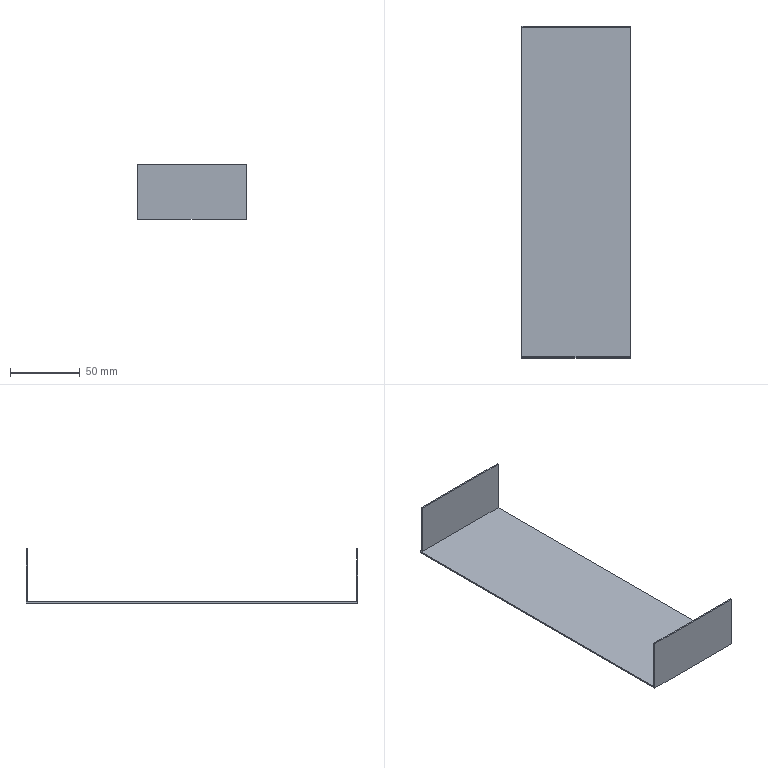Part | SolidWorks | features ICE 2, Extrusion 1 | 1 solid | 12 faces | box 78 x 238 x 39 mm | volume 24455 mm3 | plane 12
STEP:
#1=CARTESIAN_POINT('',(-38.5,118.,2.));
#2=VERTEX_POINT('',#1);
#3=CARTESIAN_POINT('',(-38.5,119.,2.));
#4=VERTEX_POINT('',#3);
#5=CARTESIAN_POINT('',(-38.5,118.,2.));
#6=DIRECTION('',(0.,1.,0.));
#7=VECTOR('',#6,1000.);
#8=LINE('',#5,#7);
#9=EDGE_CURVE('',#2,#4,#8,.T.);
#10=ORIENTED_EDGE('',*,*,#9,.F.);
#11=CARTESIAN_POINT('',(-38.5,118.,39.));
#12=VERTEX_POINT('',#11);
#13=CARTESIAN_POINT('',(-38.5,118.,39.));
#14=DIRECTION('',(0.,0.,-1.));
#15=VECTOR('',#14,1000.);
#16=LINE('',#13,#15);
#17=EDGE_CURVE('',#12,#2,#16,.T.);
#18=ORIENTED_EDGE('',*,*,#17,.F.);
#19=CARTESIAN_POINT('',(-38.5,119.,39.));
#20=VERTEX_POINT('',#19);
#21=CARTESIAN_POINT('',(-38.5,119.,39.));
#22=DIRECTION('',(0.,-1.,0.));
#23=VECTOR('',#22,1000.);
#24=LINE('',#21,#23);
#25=EDGE_CURVE('',#20,#12,#24,.T.);
#26=ORIENTED_EDGE('',*,*,#25,.F.);
#27=CARTESIAN_POINT('',(-38.5,119.,1.));
#28=DIRECTION('',(0.,0.,-1.));
#29=VECTOR('',#28,1000.);
#30=LINE('',#27,#29);
#31=EDGE_CURVE('',#20,#4,#30,.T.);
#32=ORIENTED_EDGE('',*,*,#31,.T.);
#33=EDGE_LOOP('',(#10,#18,#26,#32));
#34=FACE_OUTER_BOUND('',#33,.T.);
#35=CARTESIAN_POINT('',(-38.5,119.,1.));
#36=DIRECTION('',(1.,0.,0.));
#37=DIRECTION('',(0.,1.,0.));
#38=AXIS2_PLACEMENT_3D('',#35,#36,#37);
#39=PLANE('',#38);
#40=ADVANCED_FACE('',(#34),#39,.F.);
#41=CARTESIAN_POINT('',(-39.5,118.,1.));
#42=VERTEX_POINT('',#41);
#43=CARTESIAN_POINT('',(38.5,118.,1.));
#44=VERTEX_POINT('',#43);
#45=CARTESIAN_POINT('',(-38.5,118.,1.));
#46=DIRECTION('',(1.,0.,0.));
#47=VECTOR('',#46,1000.);
#48=LINE('',#45,#47);
#49=EDGE_CURVE('',#42,#44,#48,.T.);
#50=ORIENTED_EDGE('',*,*,#49,.F.);
#51=CARTESIAN_POINT('',(-39.5,-118.,1.));
#52=VERTEX_POINT('',#51);
#53=CARTESIAN_POINT('',(-39.5,-118.,1.));
#54=DIRECTION('',(0.,1.,0.));
#55=VECTOR('',#54,1000.);
#56=LINE('',#53,#55);
#57=EDGE_CURVE('',#52,#42,#56,.T.);
#58=ORIENTED_EDGE('',*,*,#57,.F.);
#59=CARTESIAN_POINT('',(38.5,-118.,1.));
#60=VERTEX_POINT('',#59);
#61=CARTESIAN_POINT('',(-38.5,-118.,1.));
#62=DIRECTION('',(-1.,0.,0.));
#63=VECTOR('',#62,1000.);
#64=LINE('',#61,#63);
#65=EDGE_CURVE('',#60,#52,#64,.T.);
#66=ORIENTED_EDGE('',*,*,#65,.F.);
#67=CARTESIAN_POINT('',(38.5,119.,1.));
#68=DIRECTION('',(0.,1.,0.));
#69=VECTOR('',#68,1000.);
#70=LINE('',#67,#69);
#71=EDGE_CURVE('',#60,#44,#70,.T.);
#72=ORIENTED_EDGE('',*,*,#71,.T.);
#73=EDGE_LOOP('',(#50,#58,#66,#72));
#74=FACE_OUTER_BOUND('',#73,.T.);
#75=CARTESIAN_POINT('',(0.,0.,1.));
#76=DIRECTION('',(0.,0.,1.));
#77=DIRECTION('',(1.,0.,0.));
#78=AXIS2_PLACEMENT_3D('',#75,#76,#77);
#79=PLANE('',#78);
#80=ADVANCED_FACE('',(#74),#79,.T.);
#81=CARTESIAN_POINT('',(38.5,-119.,0.));
#82=VERTEX_POINT('',#81);
#83=CARTESIAN_POINT('',(38.5,119.,0.));
#84=VERTEX_POINT('',#83);
#85=CARTESIAN_POINT('',(38.5,119.,0.));
#86=DIRECTION('',(0.,1.,0.));
#87=VECTOR('',#86,1000.);
#88=LINE('',#85,#87);
#89=EDGE_CURVE('',#82,#84,#88,.T.);
#90=ORIENTED_EDGE('',*,*,#89,.T.);
#91=CARTESIAN_POINT('',(38.5,119.,39.));
#92=VERTEX_POINT('',#91);
#93=CARTESIAN_POINT('',(38.5,119.,1.));
#94=DIRECTION('',(0.,0.,-1.));
#95=VECTOR('',#94,1000.);
#96=LINE('',#93,#95);
#97=EDGE_CURVE('',#92,#84,#96,.T.);
#98=ORIENTED_EDGE('',*,*,#97,.F.);
#99=CARTESIAN_POINT('',(38.5,118.,39.));
#100=VERTEX_POINT('',#99);
#101=CARTESIAN_POINT('',(38.5,119.,39.));
#102=DIRECTION('',(0.,1.,0.));
#103=VECTOR('',#102,1000.);
#104=LINE('',#101,#103);
#105=EDGE_CURVE('',#100,#92,#104,.T.);
#106=ORIENTED_EDGE('',*,*,#105,.F.);
#107=CARTESIAN_POINT('',(38.5,118.,39.));
#108=DIRECTION('',(0.,0.,-1.));
#109=VECTOR('',#108,1000.);
#110=LINE('',#107,#109);
#111=EDGE_CURVE('',#100,#44,#110,.T.);
#112=ORIENTED_EDGE('',*,*,#111,.T.);
#113=ORIENTED_EDGE('',*,*,#71,.F.);
#114=CARTESIAN_POINT('',(38.5,-118.,39.));
#115=VERTEX_POINT('',#114);
#116=CARTESIAN_POINT('',(38.5,-118.,39.));
#117=DIRECTION('',(0.,0.,-1.));
#118=VECTOR('',#117,1000.);
#119=LINE('',#116,#118);
#120=EDGE_CURVE('',#115,#60,#119,.T.);
#121=ORIENTED_EDGE('',*,*,#120,.F.);
#122=CARTESIAN_POINT('',(38.5,-119.,39.));
#123=VERTEX_POINT('',#122);
#124=CARTESIAN_POINT('',(38.5,-119.,39.));
#125=DIRECTION('',(0.,1.,0.));
#126=VECTOR('',#125,1000.);
#127=LINE('',#124,#126);
#128=EDGE_CURVE('',#123,#115,#127,.T.);
#129=ORIENTED_EDGE('',*,*,#128,.F.);
#130=CARTESIAN_POINT('',(38.5,-119.,1.));
#131=DIRECTION('',(0.,0.,-1.));
#132=VECTOR('',#131,1000.);
#133=LINE('',#130,#132);
#134=EDGE_CURVE('',#123,#82,#133,.T.);
#135=ORIENTED_EDGE('',*,*,#134,.T.);
#136=EDGE_LOOP('',(#90,#98,#106,#112,#113,#121,#129,#135));
#137=FACE_OUTER_BOUND('',#136,.T.);
#138=CARTESIAN_POINT('',(38.5,119.,1.));
#139=DIRECTION('',(-1.,0.,0.));
#140=DIRECTION('',(0.,-1.,0.));
#141=AXIS2_PLACEMENT_3D('',#138,#139,#140);
#142=PLANE('',#141);
#143=ADVANCED_FACE('',(#137),#142,.F.);
#144=CARTESIAN_POINT('',(-39.5,119.,0.));
#145=VERTEX_POINT('',#144);
#146=CARTESIAN_POINT('',(-38.5,119.,0.));
#147=DIRECTION('',(-1.,0.,0.));
#148=VECTOR('',#147,1000.);
#149=LINE('',#146,#148);
#150=EDGE_CURVE('',#84,#145,#149,.T.);
#151=ORIENTED_EDGE('',*,*,#150,.T.);
#152=CARTESIAN_POINT('',(-39.5,119.,2.));
#153=VERTEX_POINT('',#152);
#154=CARTESIAN_POINT('',(-39.5,119.,2.));
#155=DIRECTION('',(0.,0.,-1.));
#156=VECTOR('',#155,1000.);
#157=LINE('',#154,#156);
#158=EDGE_CURVE('',#153,#145,#157,.T.);
#159=ORIENTED_EDGE('',*,*,#158,.F.);
#160=CARTESIAN_POINT('',(-39.5,119.,2.));
#161=DIRECTION('',(1.,0.,0.));
#162=VECTOR('',#161,1000.);
#163=LINE('',#160,#162);
#164=EDGE_CURVE('',#153,#4,#163,.T.);
#165=ORIENTED_EDGE('',*,*,#164,.T.);
#166=ORIENTED_EDGE('',*,*,#31,.F.);
#167=CARTESIAN_POINT('',(-38.5,119.,39.));
#168=DIRECTION('',(-1.,0.,0.));
#169=VECTOR('',#168,1000.);
#170=LINE('',#167,#169);
#171=EDGE_CURVE('',#92,#20,#170,.T.);
#172=ORIENTED_EDGE('',*,*,#171,.F.);
#173=ORIENTED_EDGE('',*,*,#97,.T.);
#174=EDGE_LOOP('',(#151,#159,#165,#166,#172,#173));
#175=FACE_OUTER_BOUND('',#174,.T.);
#176=CARTESIAN_POINT('',(-38.5,119.,1.));
#177=DIRECTION('',(0.,-1.,0.));
#178=DIRECTION('',(0.,0.,-1.));
#179=AXIS2_PLACEMENT_3D('',#176,#177,#178);
#180=PLANE('',#179);
#181=ADVANCED_FACE('',(#175),#180,.F.);
#182=CARTESIAN_POINT('',(-39.5,-119.,0.));
#183=VERTEX_POINT('',#182);
#184=CARTESIAN_POINT('',(-38.5,-119.,0.));
#185=DIRECTION('',(1.,0.,0.));
#186=VECTOR('',#185,1000.);
#187=LINE('',#184,#186);
#188=EDGE_CURVE('',#183,#82,#187,.T.);
#189=ORIENTED_EDGE('',*,*,#188,.T.);
#190=ORIENTED_EDGE('',*,*,#134,.F.);
#191=CARTESIAN_POINT('',(-39.5,-119.,39.));
#192=VERTEX_POINT('',#191);
#193=CARTESIAN_POINT('',(-38.5,-119.,39.));
#194=DIRECTION('',(1.,0.,0.));
#195=VECTOR('',#194,1000.);
#196=LINE('',#193,#195);
#197=EDGE_CURVE('',#192,#123,#196,.T.);
#198=ORIENTED_EDGE('',*,*,#197,.F.);
#199=CARTESIAN_POINT('',(-39.5,-119.,0.));
#200=DIRECTION('',(0.,0.,1.));
#201=VECTOR('',#200,1000.);
#202=LINE('',#199,#201);
#203=EDGE_CURVE('',#183,#192,#202,.T.);
#204=ORIENTED_EDGE('',*,*,#203,.F.);
#205=EDGE_LOOP('',(#189,#190,#198,#204));
#206=FACE_OUTER_BOUND('',#205,.T.);
#207=CARTESIAN_POINT('',(-38.5,-119.,1.));
#208=DIRECTION('',(0.,1.,0.));
#209=DIRECTION('',(0.,0.,1.));
#210=AXIS2_PLACEMENT_3D('',#207,#208,#209);
#211=PLANE('',#210);
#212=ADVANCED_FACE('',(#206),#211,.F.);
#213=ORIENTED_EDGE('',*,*,#89,.F.);
#214=ORIENTED_EDGE('',*,*,#188,.F.);
#215=CARTESIAN_POINT('',(-39.5,119.,0.));
#216=DIRECTION('',(0.,-1.,0.));
#217=VECTOR('',#216,1000.);
#218=LINE('',#215,#217);
#219=EDGE_CURVE('',#145,#183,#218,.T.);
#220=ORIENTED_EDGE('',*,*,#219,.F.);
#221=ORIENTED_EDGE('',*,*,#150,.F.);
#222=EDGE_LOOP('',(#213,#214,#220,#221));
#223=FACE_OUTER_BOUND('',#222,.T.);
#224=CARTESIAN_POINT('',(0.,0.,0.));
#225=DIRECTION('',(0.,0.,1.));
#226=DIRECTION('',(1.,0.,0.));
#227=AXIS2_PLACEMENT_3D('',#224,#225,#226);
#228=PLANE('',#227);
#229=ADVANCED_FACE('',(#223),#228,.F.);
#230=ORIENTED_EDGE('',*,*,#49,.T.);
#231=ORIENTED_EDGE('',*,*,#111,.F.);
#232=CARTESIAN_POINT('',(-38.5,118.,39.));
#233=DIRECTION('',(1.,0.,0.));
#234=VECTOR('',#233,1000.);
#235=LINE('',#232,#234);
#236=EDGE_CURVE('',#12,#100,#235,.T.);
#237=ORIENTED_EDGE('',*,*,#236,.F.);
#238=ORIENTED_EDGE('',*,*,#17,.T.);
#239=CARTESIAN_POINT('',(-39.5,118.,2.));
#240=VERTEX_POINT('',#239);
#241=CARTESIAN_POINT('',(-39.5,118.,2.));
#242=DIRECTION('',(1.,0.,0.));
#243=VECTOR('',#242,1000.);
#244=LINE('',#241,#243);
#245=EDGE_CURVE('',#240,#2,#244,.T.);
#246=ORIENTED_EDGE('',*,*,#245,.F.);
#247=CARTESIAN_POINT('',(-39.5,118.,1.));
#248=DIRECTION('',(0.,0.,1.));
#249=VECTOR('',#248,1000.);
#250=LINE('',#247,#249);
#251=EDGE_CURVE('',#42,#240,#250,.T.);
#252=ORIENTED_EDGE('',*,*,#251,.F.);
#253=EDGE_LOOP('',(#230,#231,#237,#238,#246,#252));
#254=FACE_OUTER_BOUND('',#253,.T.);
#255=CARTESIAN_POINT('',(-38.5,118.,39.));
#256=DIRECTION('',(0.,1.,0.));
#257=DIRECTION('',(0.,0.,1.));
#258=AXIS2_PLACEMENT_3D('',#255,#256,#257);
#259=PLANE('',#258);
#260=ADVANCED_FACE('',(#254),#259,.F.);
#261=ORIENTED_EDGE('',*,*,#25,.T.);
#262=ORIENTED_EDGE('',*,*,#236,.T.);
#263=ORIENTED_EDGE('',*,*,#105,.T.);
#264=ORIENTED_EDGE('',*,*,#171,.T.);
#265=EDGE_LOOP('',(#261,#262,#263,#264));
#266=FACE_OUTER_BOUND('',#265,.T.);
#267=CARTESIAN_POINT('',(0.,0.,39.));
#268=DIRECTION('',(0.,0.,1.));
#269=DIRECTION('',(1.,0.,0.));
#270=AXIS2_PLACEMENT_3D('',#267,#268,#269);
#271=PLANE('',#270);
#272=ADVANCED_FACE('',(#266),#271,.T.);
#273=ORIENTED_EDGE('',*,*,#65,.T.);
#274=CARTESIAN_POINT('',(-39.5,-118.,39.));
#275=VERTEX_POINT('',#274);
#276=CARTESIAN_POINT('',(-39.5,-118.,39.));
#277=DIRECTION('',(0.,0.,-1.));
#278=VECTOR('',#277,1000.);
#279=LINE('',#276,#278);
#280=EDGE_CURVE('',#275,#52,#279,.T.);
#281=ORIENTED_EDGE('',*,*,#280,.F.);
#282=CARTESIAN_POINT('',(-38.5,-118.,39.));
#283=DIRECTION('',(-1.,0.,0.));
#284=VECTOR('',#283,1000.);
#285=LINE('',#282,#284);
#286=EDGE_CURVE('',#115,#275,#285,.T.);
#287=ORIENTED_EDGE('',*,*,#286,.F.);
#288=ORIENTED_EDGE('',*,*,#120,.T.);
#289=EDGE_LOOP('',(#273,#281,#287,#288));
#290=FACE_OUTER_BOUND('',#289,.T.);
#291=CARTESIAN_POINT('',(-38.5,-118.,39.));
#292=DIRECTION('',(0.,-1.,0.));
#293=DIRECTION('',(0.,0.,-1.));
#294=AXIS2_PLACEMENT_3D('',#291,#292,#293);
#295=PLANE('',#294);
#296=ADVANCED_FACE('',(#290),#295,.F.);
#297=ORIENTED_EDGE('',*,*,#197,.T.);
#298=ORIENTED_EDGE('',*,*,#128,.T.);
#299=ORIENTED_EDGE('',*,*,#286,.T.);
#300=CARTESIAN_POINT('',(-39.5,-119.,39.));
#301=DIRECTION('',(0.,1.,0.));
#302=VECTOR('',#301,1000.);
#303=LINE('',#300,#302);
#304=EDGE_CURVE('',#192,#275,#303,.T.);
#305=ORIENTED_EDGE('',*,*,#304,.F.);
#306=EDGE_LOOP('',(#297,#298,#299,#305));
#307=FACE_OUTER_BOUND('',#306,.T.);
#308=CARTESIAN_POINT('',(0.,0.,39.));
#309=DIRECTION('',(0.,0.,1.));
#310=DIRECTION('',(1.,0.,0.));
#311=AXIS2_PLACEMENT_3D('',#308,#309,#310);
#312=PLANE('',#311);
#313=ADVANCED_FACE('',(#307),#312,.T.);
#314=ORIENTED_EDGE('',*,*,#9,.T.);
#315=ORIENTED_EDGE('',*,*,#164,.F.);
#316=CARTESIAN_POINT('',(-39.5,118.,2.));
#317=DIRECTION('',(0.,1.,0.));
#318=VECTOR('',#317,1000.);
#319=LINE('',#316,#318);
#320=EDGE_CURVE('',#240,#153,#319,.T.);
#321=ORIENTED_EDGE('',*,*,#320,.F.);
#322=ORIENTED_EDGE('',*,*,#245,.T.);
#323=EDGE_LOOP('',(#314,#315,#321,#322));
#324=FACE_OUTER_BOUND('',#323,.T.);
#325=CARTESIAN_POINT('',(-39.5,118.,2.));
#326=DIRECTION('',(0.,0.,-1.));
#327=DIRECTION('',(-1.,0.,0.));
#328=AXIS2_PLACEMENT_3D('',#325,#326,#327);
#329=PLANE('',#328);
#330=ADVANCED_FACE('',(#324),#329,.F.);
#331=ORIENTED_EDGE('',*,*,#320,.T.);
#332=ORIENTED_EDGE('',*,*,#158,.T.);
#333=ORIENTED_EDGE('',*,*,#219,.T.);
#334=ORIENTED_EDGE('',*,*,#203,.T.);
#335=ORIENTED_EDGE('',*,*,#304,.T.);
#336=ORIENTED_EDGE('',*,*,#280,.T.);
#337=ORIENTED_EDGE('',*,*,#57,.T.);
#338=ORIENTED_EDGE('',*,*,#251,.T.);
#339=EDGE_LOOP('',(#331,#332,#333,#334,#335,#336,#337,#338));
#340=FACE_OUTER_BOUND('',#339,.T.);
#341=CARTESIAN_POINT('',(-39.5,0.,0.));
#342=DIRECTION('',(-1.,0.,0.));
#343=DIRECTION('',(0.,0.,1.));
#344=AXIS2_PLACEMENT_3D('',#341,#342,#343);
#345=PLANE('',#344);
#346=ADVANCED_FACE('',(#340),#345,.T.);
#347=CLOSED_SHELL('',(#40,#80,#143,#181,#212,#229,#260,#272,#296,#313,#330,#346));
#348=MANIFOLD_SOLID_BREP('',#347);
#349=CARTESIAN_POINT('',(0.,0.,0.));
#350=DIRECTION('',(0.,0.,1.));
#351=DIRECTION('',(1.,0.,0.));
#352=AXIS2_PLACEMENT_3D('',#349,#350,#351);
#353=(LENGTH_UNIT()NAMED_UNIT(*)SI_UNIT(.MILLI.,.METRE.));
#354=UNCERTAINTY_MEASURE_WITH_UNIT(LENGTH_MEASURE(0.00001),#353,'','');
#355=(NAMED_UNIT(*)PLANE_ANGLE_UNIT()SI_UNIT($,.RADIAN.));
#356=(NAMED_UNIT(*)SI_UNIT($,.STERADIAN.)SOLID_ANGLE_UNIT());
#357=(GEOMETRIC_REPRESENTATION_CONTEXT(3)GLOBAL_UNCERTAINTY_ASSIGNED_CONTEXT((#354))GLOBAL_UNIT_ASSIGNED_CONTEXT((#353,#355,#356))REPRESENTATION_CONTEXT('',''));
#358=ADVANCED_BREP_SHAPE_REPRESENTATION('',(#348,#352),#357);